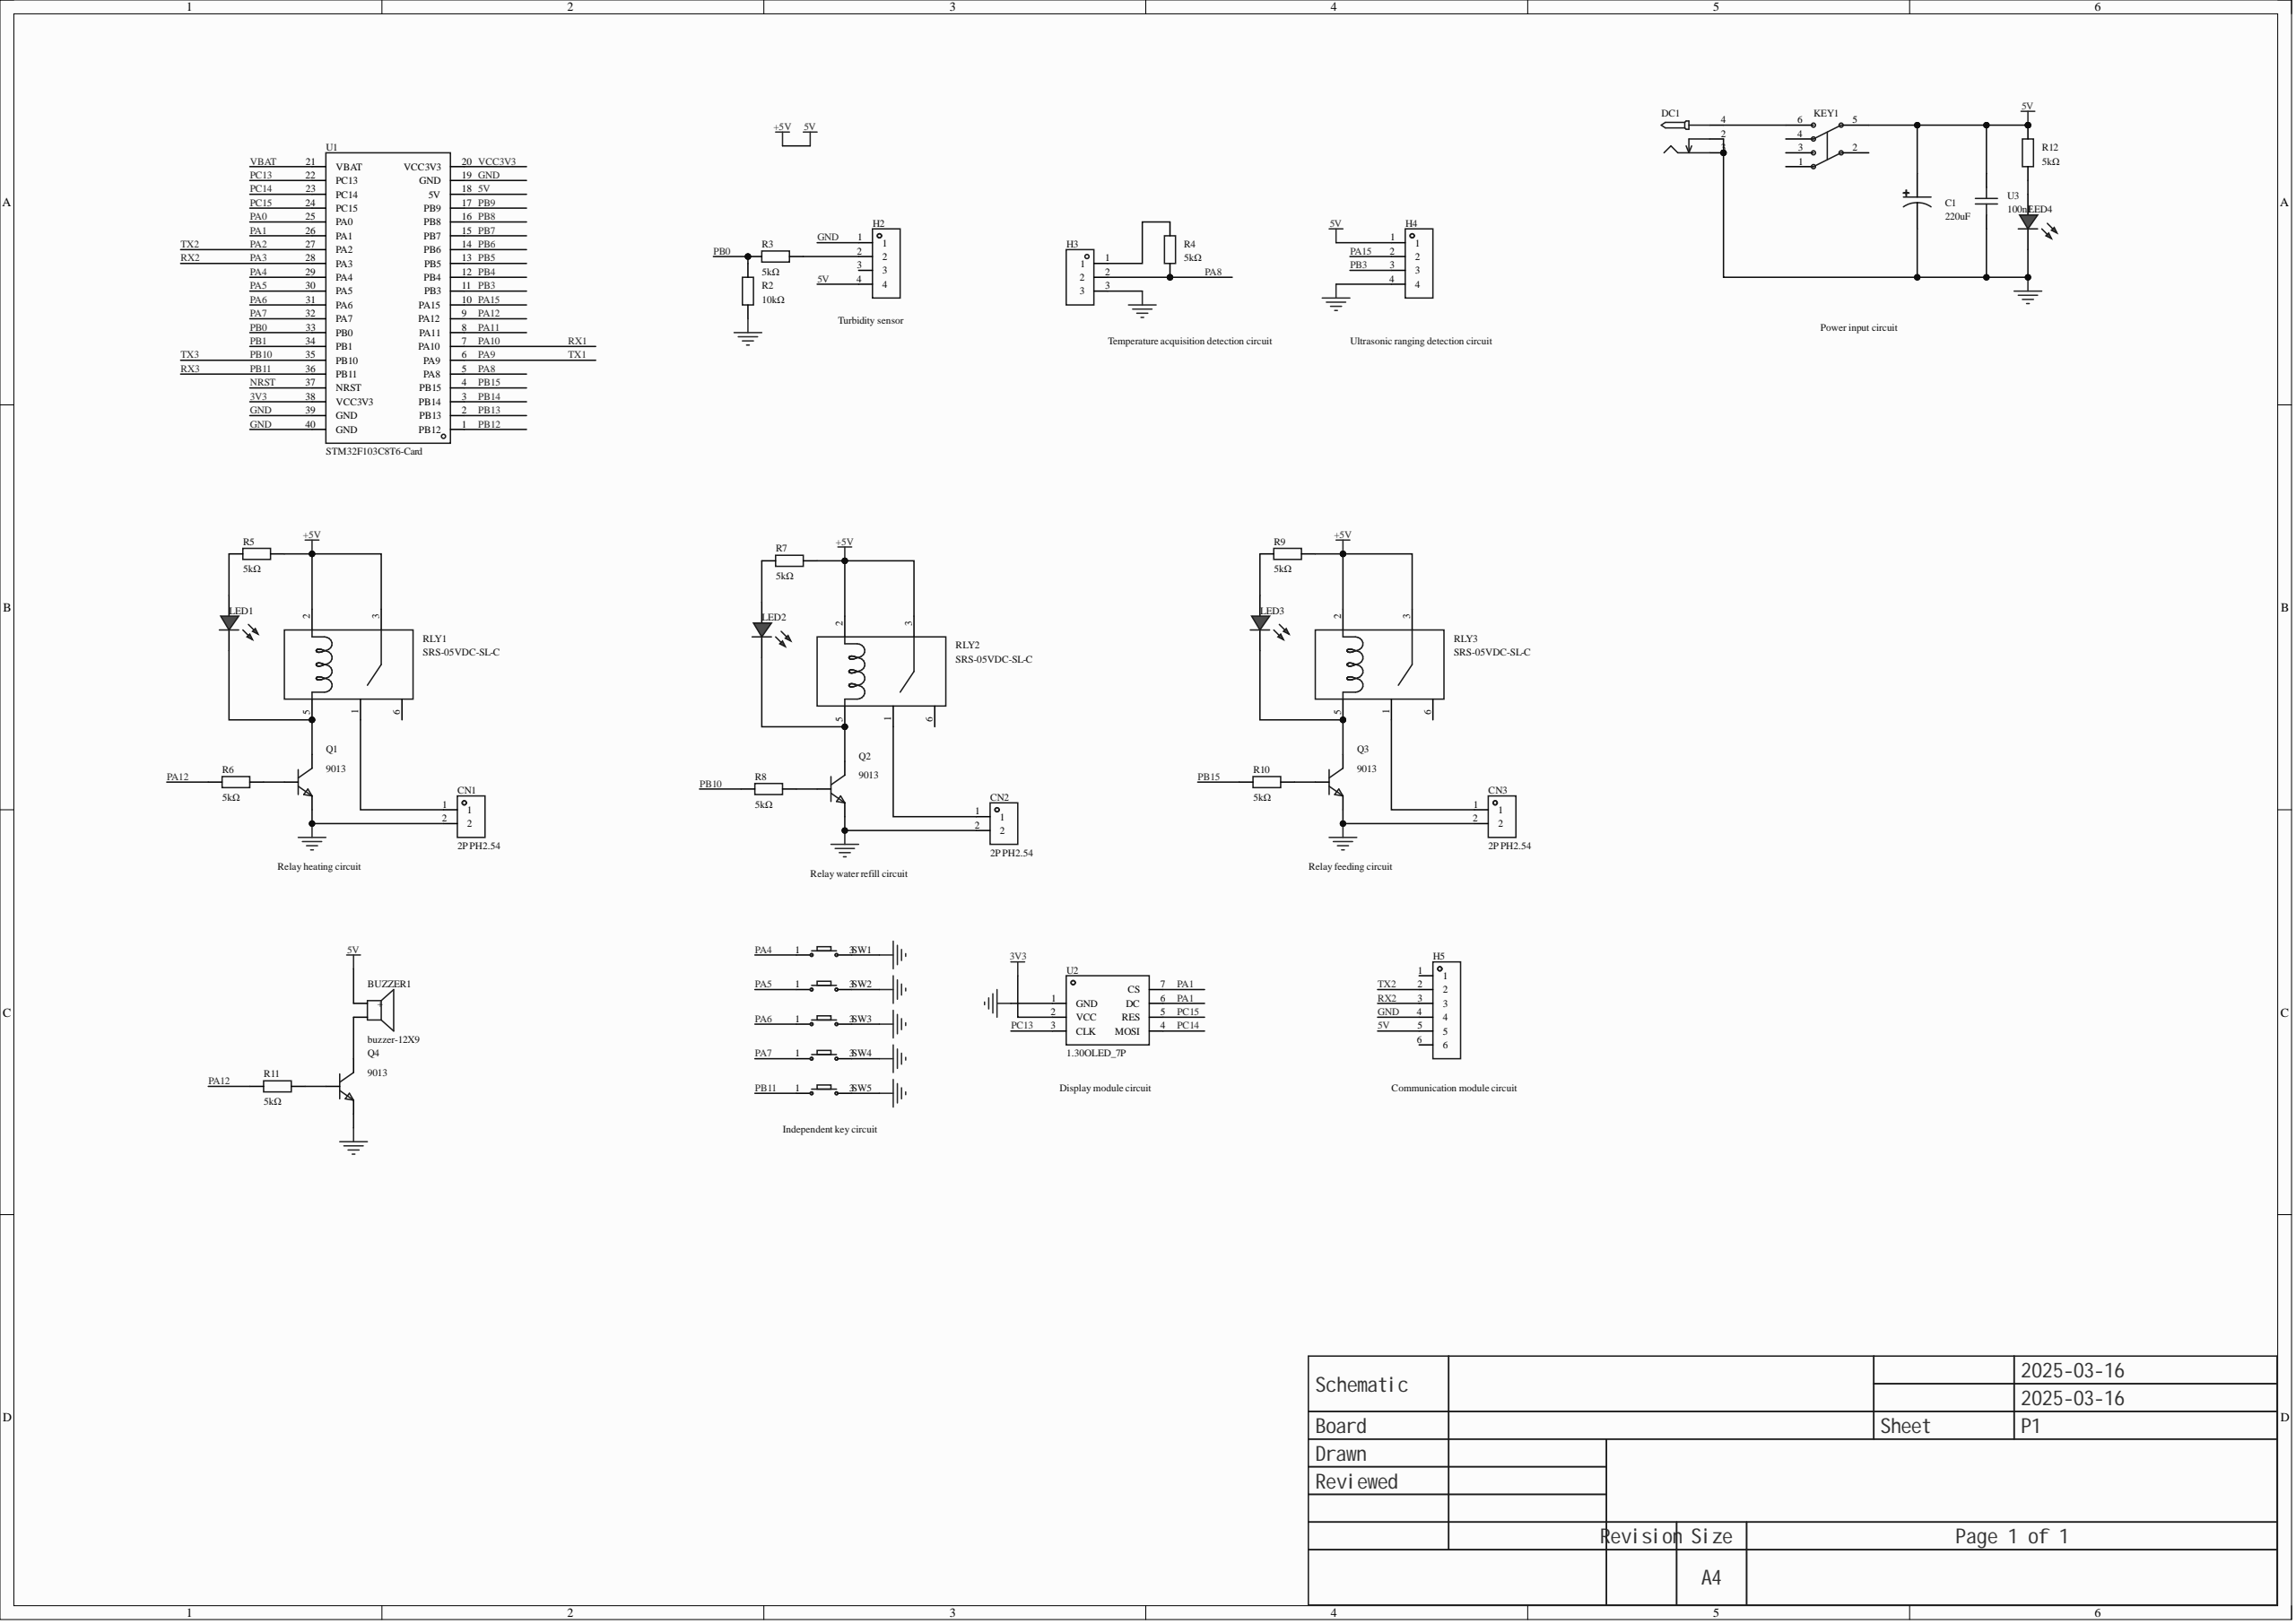Circuit board | Altium Designer | 41 parts | 39 nets
Bill of materials:
Comment,Description,Designator,Footprint,LibRef,Quantity
"buzzer-12X9","","BUZZER1","BUZ-TH_BD12.0-P7.60-D0.6-FD","buzzer-12X9","1"
"220uF","Capacitance: 220uF; Tolerance: ±20%; Rated voltage: 10V; Ripple current: -; ESR: -;","C1","CAP-TH_BD6.3-P2.50-D1.0-FD","SS2271AMD052RB","1"
"2P PH2.54","","CN1, CN2, CN3","CONN-TH_2P-P2.54_HDR2","2P PH2.54","3"
"","","DC1","DC-2.0","DC-005_2.0","1"
"","","H2, H4","HDR-TH_4P-P2.54-V-F","HDR-F_2.54_1x4P","2"
"","","H3","HDR-TH_3P-P2.54-V-F","HDR-F_2.54_1x3P","1"
"","","H5","HDR-TH_6P-P2.54-V-F","HDR-F_2.54_1x6P","1"
"Non-latching switch 8.5×8.5 silent","6 pins, 8.5×8.5","KEY1","SW-TH_6P-L8.5-W8.5-P2.54","无自锁开关 8.5×8.5 无声","1"
"","","LED1, LED2, LED3, LED4","LED-TH_5mm","LED_TH-R_5mm","4"
"9013","Transistor type: NPN; Collector current (Ic): 500mA; Collector-emitter breakdown voltage (Vceo): 20V; Power (Pd): 625mW;","Q1, Q2, Q3, Q4","TO-92-3_L4.8-W3.7-P2.54-R","9013","4"
"10kΩ","","R2","Res_1/4W","Res_AXIAL-1/4W","1"
"5kΩ","","R3, R4, R5, R6, R7, R8, R9, R10, R11, R12","Res_1/4W","Res_AXIAL-1/4W","10"
"SRS-05VDC-SL-C","","RLY1, RLY2, RLY3","RELAY-TH_SRS-05VDC-SL-C","SRS-05VDC-SL-C","3"
"","","SW1, SW2, SW3, SW4, SW5","SW-TH_4P-L6.0-W6.0-P4.50-LS6.5","Key_TH_6x6x6","5"
"STM32F103C8T6-Card","","U1","CONN-TH_L53.3-W22.9_STM32F103C8T6-CARD","STM32F103C8T6-Card","1"
"1.30OLED_7P","","U2","LCD-TH_7P-P2.54_1.30OLED_7P","1.30OLED_7P","1"
"100nF","","U3","CAP-TH_L5.0-W2.5-P5.00-D1.0","100nF","1"
Netlist (Protel format):
[
BUZZER1
BUZ-TH_BD12.0-P7.60-D0.6-FD
buzzer-12X9



]
[
C1
CAP-TH_BD6.3-P2.50-D1.0-FD
220uF



]
[
CN1
CONN-TH_2P-P2.54_HDR2
2P PH2.54



]
[
CN2
CONN-TH_2P-P2.54_HDR2
2P PH2.54



]
[
CN3
CONN-TH_2P-P2.54_HDR2
2P PH2.54



]
[
DC1
DC-2.0




]
[
H2
HDR-TH_4P-P2.54-V-F




]
[
H3
HDR-TH_3P-P2.54-V-F




]
[
H4
HDR-TH_4P-P2.54-V-F




]
[
H5
HDR-TH_6P-P2.54-V-F




]
[
KEY1
SW-TH_6P-L8.5-W8.5-P2.54
Non-latching switch 8.5×8.5 silent



]
[
LED1
LED-TH_5mm




]
[
LED2
LED-TH_5mm




]
[
LED3
LED-TH_5mm




]
[
LED4
LED-TH_5mm




]
[
Q1
TO-92-3_L4.8-W3.7-P2.54-R
9013



]
[
Q2
TO-92-3_L4.8-W3.7-P2.54-R
9013



]
[
Q3
TO-92-3_L4.8-W3.7-P2.54-R
9013



]
[
Q4
TO-92-3_L4.8-W3.7-P2.54-R
9013



]
[
R2
Res_1/4W
10kΩ



]
[
R3
Res_1/4W
5kΩ



]
[
R4
Res_1/4W
5kΩ



]
[
R5
Res_1/4W
5kΩ



]
[
R6
Res_1/4W
5kΩ



]
[
R7
Res_1/4W
5kΩ



]
[
R8
Res_1/4W
5kΩ



]
[
R9
Res_1/4W
5kΩ



]
[
R10
Res_1/4W
5kΩ



]
[
R11
Res_1/4W
5kΩ



]
[
R12
Res_1/4W
5kΩ



]
[
RLY1
RELAY-TH_SRS-05VDC-SL-C
SRS-05VDC-SL-C



]
[
RLY2
RELAY-TH_SRS-05VDC-SL-C
SRS-05VDC-SL-C



]
[
RLY3
RELAY-TH_SRS-05VDC-SL-C
SRS-05VDC-SL-C



]
[
SW1
SW-TH_4P-L6.0-W6.0-P4.50-LS6.5




]
[
SW2
SW-TH_4P-L6.0-W6.0-P4.50-LS6.5




]
[
SW3
SW-TH_4P-L6.0-W6.0-P4.50-LS6.5




]
[
SW4
SW-TH_4P-L6.0-W6.0-P4.50-LS6.5




]
[
SW5
SW-TH_4P-L6.0-W6.0-P4.50-LS6.5




]
[
U1
CONN-TH_L53.3-W22.9_STM32F103C8T6-CARD
STM32F103C8T6-Card



]
[
U2
LCD-TH_7P-P2.54_1.30OLED_7P
1.30OLED_7P



]
[
U3
CAP-TH_L5.0-W2.5-P5.00-D1.0
100nF



]
(
PC15
U1-24
U2-5
)
(
PC14
U1-23
U2-4
)
(
PC13
U1-22
U2-3
)
(
PB15
R10-1
U1-4
)
(
PB11
SW5-1
U1-36
)
(
PB10
R8-1
U1-35
)
(
PB3
H4-3
U1-11
)
(
PB0
R2-2
R3-1
U1-33
)
(
PA15
H4-2
U1-10
)
(
PA12
R6-1
R11-1
U1-9
)
(
PA8
H3-2
R4-1
U1-5
)
(
PA7
SW4-1
U1-32
)
(
PA6
SW3-1
U1-31
)
(
PA5
SW2-1
U1-30
)
(
PA4
SW1-1
U1-29
)
(
PA3
H5-3
U1-28
)
(
PA2
H5-2
U1-27
)
(
PA1
U1-26
U2-6
U2-7
)
(
NetQ4_2
Q4-2
R11-2
)
(
NetQ3_2
Q3-2
R10-2
)
(
NetQ2_2
Q2-2
R8-2
)
(
NetQ1_2
Q1-2
R6-2
)
(
NetLED4_1
LED4-1
R12-1
)
(
NetLED3_2
LED3-2
Q3-1
RLY3-5
)
(
NetLED3_1
LED3-1
R9-1
)
(
NetLED2_2
LED2-2
Q2-1
RLY2-5
)
(
NetLED2_1
LED2-1
R7-1
)
(
NetLED1_2
LED1-2
Q1-1
RLY1-5
)
(
NetLED1_1
LED1-1
R5-1
)
(
NetH3_1
H3-1
R4-2
)
(
NetH2_2
H2-2
R3-2
)
(
NetDC1_4
DC1-4
KEY1-6
)
(
NetCN3_1
CN3-1
RLY3-1
)
(
NetCN2_1
CN2-1
RLY2-1
)
(
NetCN1_1
CN1-1
RLY1-1
)
(
NetBUZZER1_2
BUZZER1-2
Q4-1
)
(
GND
C1-2
CN1-2
CN2-2
CN3-2
DC1-2
DC1-3
H2-1
H3-3
H4-4
H5-4
LED4-2
Q1-3
Q2-3
Q3-3
Q4-3
R2-1
SW1-3
SW2-3
SW3-3
SW4-3
SW5-3
U1-19
U1-39
U1-40
U2-1
U3-2
)
(
5V
BUZZER1-1
C1-1
H2-4
H4-1
H5-5
KEY1-5
R5-2
R7-2
R9-2
R12-2
RLY1-2
RLY1-3
RLY2-2
RLY2-3
RLY3-2
RLY3-3
U1-18
U3-1
)
(
3V3
U1-38
U2-2
)